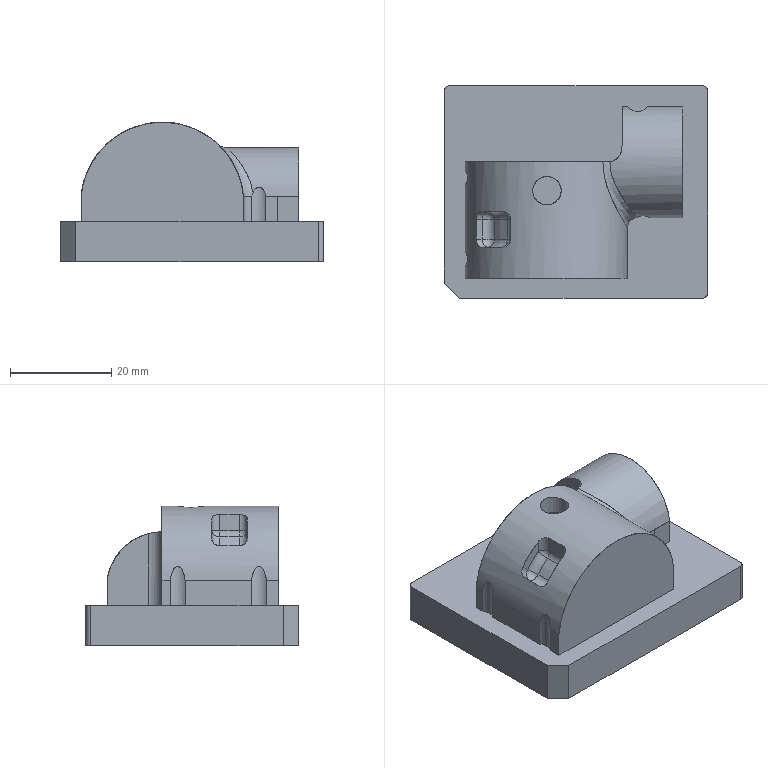NC program | PowerMill | posted with a generic post | part box 52 x 42 x 27.622 mm
Lines 35812 to 36533 of 214543:
N35909 M6
N35910 S8500 M03
N35911 G00 G90 X0.0 Y0.0
N35912 G43 Z9.8022 H3
N35913
N35914 G05 P10000 R8
N35915 X-31.7585 Y-27.2674
N35916 Z-18.62
N35917 G01 Z-19.82 F360.0
N35918 X-28.0283 Y-23.5376 F600.0
N35919 X-25.5003 Y-21.0097
N35920 X-25.7421 Y-20.7679
N35921 X-26.034 Y-20.4345
N35922 G02 X-26.4761 Y-19.7862 I4.9869 J3.8747
N35923 G02 X-26.8165 Y-19.0792 I5.3616 J3.0176
N35924 G01 X-26.9462 Y-18.7087
N35925 X-27.0478 Y-18.3294
N35926 X-27.1208 Y-17.9437
N35927 X-27.1647 Y-17.5535
N35928 X-27.1794 Y-17.1612
N35929 Y-14.7229
N35930 X-27.1661 Y-14.3483
N35931 X-27.126 Y-13.9757
N35932 X-27.0832 Y-13.7323
N35933 X-27.0299 Y-13.4909
N35934 G03 X-27.0298 Y-12.9964 I-0.9689 J0.2473
N35935 G02 X-27.1534 Y-12.257 I4.4498 J1.1234
N35936 G01 X-27.1661 Y-12.139
N35937 X-27.1794 Y-11.7644
N35938 Y1.3491
N35939 X-27.1661 Y1.7237
N35940 X-27.126 Y2.0963
N35941 X-27.0594 Y2.4652
N35942 X-27.0299 Y2.581
N35943 G03 Y3.0757 I-0.9689 J0.2473
N35944 G01 X-27.0826 Y3.3199
N35945 X-27.126 Y3.5604
N35946 X-27.1661 Y3.933
N35947 X-27.1794 Y4.3076
N35948 Y5.9414
N35949 X-27.1647 Y6.3337
N35950 X-27.1208 Y6.7239
N35951 X-27.0478 Y7.1096
N35952 X-26.9462 Y7.4889
N35953 X-26.8165 Y7.8594
N35954 G02 X-26.4952 Y8.5301 I5.2353 J-2.0955
N35955 G01 X-26.2672 Y8.8988
N35956 X-26.0341 Y9.2147
N35957 X-25.778 Y9.5123
N35958 X-25.5003 Y9.7899
N35959 X-25.2028 Y10.046
N35960 X-24.8869 Y10.2792
N35961 X-24.5544 Y10.488
N35962 X-24.2073 Y10.6715
N35963 X-23.9315 Y10.7922
N35964 X-23.6503 Y10.8995
N35965 X-24.9728 Y15.5253
N35966 X-25.4378 Y15.3924
N35967 G02 X-26.5431 Y16.2689 I-0.2386 J0.8343
N35968 G01 X-26.389 Y19.4393
N35969 G02 X-24.2172 Y21.5109 I2.1749 J-0.1058
N35970 G01 X-0.9855 Y21.5443
N35971 G02 X-0.1644 Y20.419 I0.0012 J-0.8614
N35972 G01 X-0.2657 Y20.1041
N35973 G03 X-0.77 Y17.8703 I12.1965 J-3.9269
N35974 G01 X-0.8682 Y17.1333
N35975 G02 X-2.1661 Y15.9958 I-1.2992 J0.1732
N35976 G01 X-22.4475 Y15.9761
N35977 X-22.832 Y15.9498
N35978 G03 X-24.6938 Y15.6051 I0.8699 J-9.8993
N35979 G01 X-24.9728 Y15.5253
N35980 X-23.6503 Y10.8995
N35981 X-23.4769 Y10.9581
N35982 G02 X-22.7119 Y11.1328 I1.7411 J-5.8651
N35983 G01 X-22.3218 Y11.1767
N35984 X-21.9294 Y11.1914
N35985 X2.8992
N35986 G03 X3.899 Y12.1739 I0.0 J1.0
N35987 G01 X3.9812 Y16.8798
N35988 X4.0023 Y17.2674
N35989 X4.052 Y17.6525
N35990 X4.1301 Y18.0328
N35991 X4.236 Y18.4063
N35992 X4.3692 Y18.771
N35993 X4.5291 Y19.1248
N35994 X4.7146 Y19.4659
N35995 X4.9248 Y19.7922
N35996 G02 X5.4147 Y20.3941 I4.9294 J-3.5117
N35997 G01 X5.6916 Y20.6662
N35998 X5.9878 Y20.9171
N35999 X6.3018 Y21.1455
N36000 X6.6319 Y21.35
N36001 X6.9761 Y21.5295
N36002 X7.3327 Y21.6832
N36003 X7.6996 Y21.81
N36004 X8.0749 Y21.9094
N36005 G02 X8.8424 Y22.0238 I1.2982 J-6.0795
N36006 G01 X9.2304 Y22.0381
N36007 X10.4243 Y22.0338
N36008 X10.6703 Y22.0233
N36009 X11.0623 Y21.9789
N36010 X11.45 Y21.9052
N36011 X11.8713 Y21.7884
N36012 G03 X12.5351 I0.3319 J0.9433
N36013 G01 X12.9565 Y21.9052
N36014 X13.3441 Y21.9789
N36015 X13.7362 Y22.0233
N36016 X14.1305 Y22.0381
N36017 X21.0985
N36018 X21.4909 Y22.0234
N36019 X21.881 Y21.9795
N36020 X22.2668 Y21.9065
N36021 X22.646 Y21.8049
N36022 X23.0166 Y21.6752
N36023 X23.4171 Y21.4968
N36024 X23.7235 Y21.3348
N36025 X24.056 Y21.1259
N36026 X24.3719 Y20.8927
N36027 X24.6694 Y20.6367
N36028 X24.9471 Y20.359
N36029 X25.2031 Y20.0615
N36030 X25.4363 Y19.7456
N36031 X25.6452 Y19.4131
N36032 G02 X26.0006 Y18.6635 I-4.9294 J-2.7961
N36033 G01 X26.1153 Y18.3356
N36034 X26.2169 Y17.9564
N36035 X26.2899 Y17.5706
N36036 X26.3339 Y17.1805
N36037 X26.3485 Y16.7881
N36038 Y-5.1044
N36039 X26.3338 Y-5.4968
N36040 X26.2899 Y-5.8869
N36041 X26.2169 Y-6.2727
N36042 X26.1153 Y-6.6519
N36043 X25.9856 Y-7.0225
N36044 X25.8286 Y-7.3823
N36045 X25.6452 Y-7.7294
N36046 X25.4363 Y-8.0619
N36047 X25.2031 Y-8.3778
N36048 X24.947 Y-8.6753
N36049 X24.6694 Y-8.9529
N36050 X24.3718 Y-9.2091
N36051 X24.056 Y-9.4422
N36052 X23.7235 Y-9.6511
N36053 X23.3764 Y-9.8345
N36054 X23.1798 Y-9.9203
N36055 X24.9239 Y-14.3937
N36056 X25.448 Y-14.1894
N36057 G02 X26.5446 Y-14.9628 I0.2923 J-0.7497
N36058 G01 X26.4152 Y-19.3477
N36059 G02 X24.1935 Y-21.5191 I-2.2365 J0.0661
N36060 G01 X20.5691 Y-21.5432
N36061 G02 X19.7114 Y-20.4389 I-0.0058 J0.8807
N36062 G01 X19.9263 Y-19.62
N36063 G03 X20.2939 Y-16.7253 I-10.8588 J2.8496
N36064 G01 X20.2926 Y-16.4098
N36065 G02 X21.3497 Y-15.2059 I1.2086 J0.0048
N36066 G01 X22.2848 Y-15.0878
N36067 G03 X24.7492 Y-14.4618 I-1.2987 J10.2777
N36068 G01 X24.9239 Y-14.3937
N36069 X23.1798 Y-9.9203
N36070 X23.0166 Y-9.9915
N36071 X22.646 Y-10.1212
N36072 X22.2668 Y-10.2228
N36073 G02 X21.4909 Y-10.3398 I-1.2879 J5.912
N36074 G01 X21.0985 Y-10.3544
N36075 X16.4239
N36076 G03 X15.4239 Y-11.3544 I0.0 J-1.0
N36077 G01 Y-17.1612
N36078 X15.4092 Y-17.5535
N36079 X15.3652 Y-17.9437
N36080 X15.2922 Y-18.3294
N36081 X15.1906 Y-18.7087
N36082 X15.061 Y-19.0792
N36083 X14.904 Y-19.4391
N36084 X14.7205 Y-19.7862
N36085 X14.4841 Y-20.1559
N36086 X14.2785 Y-20.4345
N36087 X14.0224 Y-20.7321
N36088 X13.7448 Y-21.0097
N36089 X13.4472 Y-21.2658
N36090 X13.1313 Y-21.499
N36091 X12.7989 Y-21.7078
N36092 X12.4518 Y-21.8913
N36093 X12.0919 Y-22.0483
N36094 X11.7214 Y-22.1779
N36095 X11.3421 Y-22.2796
N36096 X10.9564 Y-22.3526
N36097 X10.5662 Y-22.3965
N36098 X10.1739 Y-22.4112
N36099 X-21.9294
N36100 X-22.3218 Y-22.3965
N36101 X-22.7119 Y-22.3526
N36102 X-23.0977 Y-22.2796
N36103 X-23.4769 Y-22.1779
N36104 X-23.8475 Y-22.0483
N36105 X-24.2073 Y-21.8913
N36106 X-24.5544 Y-21.7078
N36107 X-24.8869 Y-21.4989
N36108 X-25.2028 Y-21.2658
N36109 X-25.5003 Y-21.0097
N36110 X-28.0283 Y-23.5376
N36111 G00 Z9.8022
N36112 G05 P0
N36113 (---------------)
N36114 ( END TOOLPATH : 粗公基准台01-基准面偏置-D10 )
N36115 (---------------)
N36116 ( START TOOLPATH : 粗公基准台01-外形侧光-D10 )
N36117 (---------------)
N36118 G00 X0.0 Y0.0 Z10.802
N36119 G05 P10000 R8
N36120 X26.0718 Y16.531
N36121 Z-8.294
N36122 G01 Z-9.494 F360.0
N36123 G03 X25.8674 Y15.4013 I1.2615 J-0.8115 F600.0
N36124 G02 X25.9777 Y14.4568 I-4.7691 J-1.0354
N36125 G01 X25.9785 Y-2.5824
N36126 G02 X25.8673 Y-3.72 I-4.8822 J-0.0969
N36127 G03 X26.0705 Y-4.8499 I1.4655 J-0.3196
N36128 G00 Z4.1556
N36129 G01 X10.7901 Y-22.1365 F10000.0
N36130 G00 Z-8.294
N36131 G01 Z-9.494 F360.0
N36132 G03 X9.6606 Y-21.9311 I-0.8127 J-1.2607 F600.0
N36133 G02 X8.6481 Y-22.0412 I-1.0309 J4.77
N36134 G01 X-5.8084
N36135 X-20.2656
N36136 G02 X-21.4209 Y-21.9306 I-0.1155 J4.8832
N36137 G03 X-22.5508 Y-22.1341 I-0.3194 J-1.4656
N36138 G00 Z4.1556
N36139 G01 X-22.5476 Y10.9144 F10000.0
N36140 G00 Z-8.294
N36141 G01 Z-9.494 F360.0
N36142 G03 X-21.4177 Y10.7107 I0.8108 J1.262 F600.0
N36143 G02 X-20.2649 Y10.8214 I1.041 J-4.7825
N36144 G01 X4.029
N36145 G03 X4.249 Y11.0376 I0.0 J0.22
N36146 G01 X4.3083 Y14.4602
N36147 G02 X4.4379 Y15.4867 I4.8792 J-0.0944
N36148 G03 X4.2539 Y16.6199 I-1.4599 J0.3445
N36149 G00 Z4.1556
N36150 G01 X26.1834 Y16.0152 F10000.0
N36151 G00 Z-8.294
N36152 G01 Z-9.494 F360.0
N36153 G03 X25.8674 Y14.9115 I1.1743 J-0.9332 F600.0
N36154 G02 X25.8977 Y14.4565 I-4.7687 J-0.5455
N36155 G01 X25.8985 Y-2.5815
N36156 G02 X25.8673 Y-3.2346 I-4.8024 J-0.0978
N36157 G03 X26.1811 Y-4.339 I1.49 J-0.1734
N36158 G00 Z4.1556
N36159 G01 X10.2699 Y-22.249 F10000.0
N36160 G00 Z-8.294
N36161 G01 Z-9.494 F360.0
N36162 G03 X9.1667 Y-21.9311 I-0.9354 J-1.1727 F600.0
N36163 G02 X8.6481 Y-21.9612 I-0.5369 J4.7706
N36164 G01 X-5.8084
N36165 X-20.2649
N36166 G02 X-20.9346 Y-21.9306 I-0.1162 J4.8032
N36167 G03 X-22.0388 Y-22.2448 I-0.1728 J-1.49
N36168 G00 Z4.1556
N36169 G01 X-22.0348 Y11.0251 F10000.0
N36170 G00 Z-8.294
N36171 G01 Z-9.494 F360.0
N36172 G03 X-20.9306 Y10.7107 I0.9316 J1.1756 F600.0
N36173 G02 X-20.2649 Y10.7414 I0.5539 J-4.7828
N36174 G01 X4.029
N36175 G03 X4.329 Y11.0362 I0.0 J0.3
N36176 G01 X4.3882 Y14.4565
N36177 G02 X4.4292 Y14.9985 I4.7991 J-0.0906
N36178 G03 X4.1335 Y16.1078 I-1.4869 J0.1977
N36179 G00 Z4.1889
N36180 G01 X15.4933 Y-12.0436 F10000.0
N36181 G00 Z-18.59
N36182 G01 Z-19.79 F360.0
N36183 G03 X15.0539 Y-13.1043 I1.0606 J-1.0607 F600.0
N36184 G01 Y-17.0386
N36185 G02 X10.197 Y-22.0411 I-4.883 J-0.1182
N36186 G01 X-5.8084 Y-22.0412
N36187 X-21.8145
N36188 G02 X-26.8075 Y-17.2968 I-0.1109 J4.8828
N36189 G02 X-26.8094 Y-14.7124 I174.8409 J1.418
N36190 G02 X-26.5991 Y-13.3087 I4.7813 J0.0012
N36191 G03 X-26.5975 Y-13.1867 I-0.2105 J0.0636
N36192 G02 X-26.8082 Y-11.8754 I4.669 J1.4225
N36193 G01 X-26.8094 Y1.292
N36194 G02 X-26.599 Y2.7658 I4.881 J0.0548
N36195 G03 X-26.5979 Y2.8926 I-0.2101 J0.0651
N36196 G02 X-26.8062 Y4.1294 I4.5302 J1.3987
N36197 G02 X-26.8094 Y5.9396 I71.3503 J1.0334
N36198 G02 X-21.8139 Y10.8214 I4.8839 J-0.0008
N36199 G01 X4.029
N36200 G03 X4.249 Y11.0376 I0.0 J0.22
N36201 G01 X4.3183 Y15.0005
N36202 X4.3495 Y16.7822
N36203 G02 X9.1644 Y21.6677 I4.8827 J0.0032
N36204 G02 X10.4603 Y21.6646 I0.5369 J-47.0757
N36205 G02 X12.1196 Y21.3052 I-0.1677 J-4.7838
N36206 G03 X12.2831 Y21.3036 I0.0838 J0.2034
N36207 G02 X14.0693 Y21.6678 I1.8403 J-4.4639
N36208 G01 X15.0759
N36209 X21.0407 Y21.6681
N36210 G02 X25.9785 Y16.7799 I0.0568 J-4.8807
N36211 G01 X25.9781 Y-5.1662
N36212 G02 X21.0394 Y-9.9844 I-4.8807 J0.0625
N36213 G01 X15.2739
N36214 G03 X15.0539 Y-10.2044 I0.0 J-0.22
N36215 G01 Y-13.1043
N36216 G03 X15.4933 Y-14.165 I1.5 J0.0
N36217 G01 X15.4133 Y-11.9768
N36218 G03 X14.9739 Y-13.0375 I1.0606 J-1.0607
N36219 G01 Y-17.038
N36220 G02 X10.197 Y-21.9611 I-4.8029 J-0.1188
N36221 G01 X-5.8084 Y-21.9612
N36222 X-21.8139
N36223 G02 X-26.7275 Y-17.2962 I-0.1115 J4.8028
N36224 G02 X-26.7294 Y-14.7147 I174.7309 J1.4187
N36225 G02 X-26.5225 Y-13.3319 I4.7004 J0.0035
N36226 G03 X-26.5204 Y-13.1655 I-0.2872 J0.0868
N36227 G02 X-26.7282 Y-11.875 I4.5906 J1.4011
N36228 G01 X-26.7294 Y1.2908
N36229 G02 X-26.5225 Y2.7421 I4.8006 J0.056
N36230 G03 X-26.5211 Y2.915 I-0.2866 J0.0888
N36231 G02 X-26.7262 Y4.1304 I4.4521 J1.3761
N36232 G02 X-26.7294 Y5.9375 I71.1887 J1.0327
N36233 G02 X-21.8139 Y10.7414 I4.8039 J0.0013
N36234 G01 X4.029
N36235 G03 X4.329 Y11.0362 I0.0 J0.3
N36236 G01 X4.3983 Y14.9991
N36237 X4.4295 Y16.7799
N36238 G02 X9.1644 Y21.5877 I4.8027 J0.0055
N36239 G02 X10.4552 Y21.5848 I0.5372 J-48.3015
N36240 G02 X12.0891 Y21.2312 I-0.1625 J-4.7033
N36241 G03 X12.3121 Y21.229 I0.1143 J0.2774
N36242 G02 X14.0693 Y21.5878 I1.8111 J-4.3881
N36243 G01 X15.0759
N36244 X21.0394 Y21.5881
N36245 G02 X25.8985 Y16.7799 I0.0581 J-4.8007
N36246 G01 X25.8982 Y-5.163
N36247 G02 X21.0394 Y-9.9044 I-4.8007 J0.0593
N36248 G01 X15.2739
N36249 G03 X14.9739 Y-10.2044 I0.0 J-0.3
N36250 G01 Y-13.0375
N36251 G03 X15.4133 Y-14.0982 I1.5 J0.0
N36252 G00 Z10.802
N36253 G05 P0
N36254 (---------------)
N36255 ( END TOOLPATH : 粗公基准台01-外形侧光-D10 )
N36256 (---------------)
N36257 ( START TOOLPATH : 粗公基准台01-基准台侧光-D10 )
N36258 (---------------)
N36259 G00 X0.0 Y0.0 Z9.8022
N36260 G05 P10000 R8
N36261 X31.5194 Y-28.9518
N36262 Z-26.52
N36263 G01 Z-27.72 F360.0
N36264 G03 X28.4722 Y-24.9877 I-1.5236 J1.982 F600.0
N36265 G01 X28.4323 Y-25.0183
N36266 X28.429 Y-25.0208
N36267 X28.4255 Y-25.023
N36268 X27.9786 Y-25.2983
N36269 X27.9758 Y-25.2999
N36270 X27.973 Y-25.3014
N36271 X27.526 Y-25.5298
N36272 X27.5229 Y-25.5313
N36273 X27.5198 Y-25.5327
N36274 X27.0728 Y-25.7144
N36275 X27.0699 Y-25.7155
N36276 X27.067 Y-25.7165
N36277 X26.62 Y-25.8596
N36278 X26.6171 Y-25.8605
N36279 X26.614 Y-25.8613
N36280 X26.1671 Y-25.9669
N36281 X26.1648 Y-25.9674
N36282 X26.1626 Y-25.9678
N36283 X25.958 Y-26.0039
N36284 X25.9565 Y-26.0042
N36285 X25.955 Y-26.0044
N36286 X25.7125 Y-26.0376
N36287 X25.7102 Y-26.0379
N36288 X25.708 Y-26.0381
N36289 X25.261 Y-26.0733
N36290 X25.2584 Y-26.0734
N36291 X25.2558 Y-26.0735
N36292 X24.8089 Y-26.08
N36293 X24.8083
N36294 X24.8077
N36295 X-23.0198
N36296 X-23.0217
N36297 X-23.0237 Y-26.0799
N36298 X-23.4706 Y-26.0581
N36299 X-23.474 Y-26.0578
N36300 X-23.4774 Y-26.0575
N36301 X-23.8725 Y-26.0045
N36302 X-23.8761 Y-26.0039
N36303 X-23.8797 Y-26.0032
N36304 X-24.3785 Y-25.8893
N36305 X-24.3823 Y-25.8883
N36306 X-24.3861 Y-25.8872
N36307 X-24.8331 Y-25.7377
N36308 X-24.8366 Y-25.7364
N36309 X-24.84 Y-25.735
N36310 X-25.2562 Y-25.5514
N36311 X-25.2599 Y-25.5497
N36312 X-25.2634 Y-25.5478
N36313 X-25.7411 Y-25.2768
N36314 X-25.7441 Y-25.2751
N36315 X-25.747 Y-25.2732
N36316 X-26.0033 Y-25.0971
N36317 X-26.0051 Y-25.0959
N36318 X-26.0068 Y-25.0945
N36319 X-26.1975 Y-24.9474
N36320 X-26.1997 Y-24.9457
N36321 X-26.2018 Y-24.9439
N36322 X-26.5393 Y-24.644
N36323 X-26.5411 Y-24.6424
N36324 X-26.5428 Y-24.6408
N36325 X-29.6706 Y-21.5119
N36326 X-29.6716 Y-21.5108
N36327 X-29.6727 Y-21.5096
N36328 X-29.7833 Y-21.3902
N36329 X-29.7848 Y-21.3884
N36330 X-29.7863 Y-21.3866
N36331 X-30.0556 Y-21.0591
N36332 X-30.0574 Y-21.0568
N36333 X-30.0591 Y-21.0545
N36334 X-30.2369 Y-20.8027
N36335 X-30.2381 Y-20.8009
N36336 X-30.2393 Y-20.7991
N36337 X-30.3619 Y-20.6039
N36338 X-30.3634 Y-20.6014
N36339 X-30.3648 Y-20.5988
N36340 X-30.6017 Y-20.1518
N36341 X-30.603 Y-20.1492
N36342 X-30.6042 Y-20.1466
N36343 X-30.6917 Y-19.9478
N36344 X-30.6925 Y-19.946
N36345 X-30.6932 Y-19.9442
N36346 X-30.7885 Y-19.6961
N36347 X-30.7895 Y-19.6933
N36348 X-30.7904 Y-19.6905
N36349 X-30.9254 Y-19.2435
N36350 X-30.9264 Y-19.2399
N36351 X-30.9272 Y-19.2364
N36352 X-31.0182 Y-18.7894
N36353 X-31.0189 Y-18.7858
N36354 X-31.0194 Y-18.7822
N36355 X-31.0689 Y-18.3352
N36356 X-31.0692 Y-18.3318
N36357 X-31.0693 Y-18.3283
N36358 X-31.08 Y-17.8813
N36359 Y-17.8804
N36360 Y-17.8794
N36361 Y19.2204
N36362 Y19.2205
N36363 X-31.0787 Y20.1145
N36364 Y20.1168
N36365 X-31.0786 Y20.1191
N36366 X-31.052 Y20.5661
N36367 X-31.0518 Y20.5688
N36368 X-31.0514 Y20.5716
N36369 X-30.9937 Y21.0186
N36370 X-30.9932 Y21.0218
N36371 X-30.9926 Y21.025
N36372 X-30.8977 Y21.4719
N36373 X-30.897 Y21.4748
N36374 X-30.8963 Y21.4775
N36375 X-30.767 Y21.9245
N36376 X-30.766 Y21.9276
N36377 X-30.7649 Y21.9306
N36378 X-30.5958 Y22.3776
N36379 X-30.5945 Y22.3807
N36380 X-30.5932 Y22.3837
N36381 X-30.3803 Y22.8307
N36382 X-30.3788 Y22.8336
N36383 X-30.3772 Y22.8365
N36384 X-30.1168 Y23.2835
N36385 X-30.1149 Y23.2866
N36386 X-30.1129 Y23.2896
N36387 X-29.7948 Y23.7366
N36388 X-29.7924 Y23.7398
N36389 X-29.7899 Y23.7429
N36390 X-29.3378 Y24.2601
N36391 X-29.3348 Y24.2633
N36392 X-29.3316 Y24.2664
N36393 X-28.9198 Y24.6432
N36394 X-28.9173 Y24.6455
N36395 X-28.9146 Y24.6476
N36396 X-28.4323 Y25.0183
N36397 X-28.429 Y25.0208
N36398 X-28.4255 Y25.023
N36399 X-27.9786 Y25.2983
N36400 X-27.9758 Y25.2999
N36401 X-27.973 Y25.3014
N36402 X-27.526 Y25.5298
N36403 X-27.5229 Y25.5313
N36404 X-27.5198 Y25.5327
N36405 X-27.0728 Y25.7144
N36406 X-27.0699 Y25.7155
N36407 X-27.067 Y25.7165
N36408 X-26.62 Y25.8596
N36409 X-26.6171 Y25.8605
N36410 X-26.614 Y25.8613
N36411 X-26.167 Y25.9669
N36412 X-26.164 Y25.9675
N36413 X-26.1609 Y25.9681
N36414 X-25.7139 Y26.0374
N36415 X-25.711 Y26.0378
N36416 X-25.708 Y26.0381
N36417 X-25.261 Y26.0733
N36418 X-25.2584 Y26.0735
N36419 X-25.2558
N36420 X-24.8089 Y26.08
N36421 X-24.8083
N36422 X-24.8077
N36423 X0.0
N36424 X24.8077
N36425 X24.8083
N36426 X24.8089
N36427 X25.2558 Y26.0735
N36428 X25.2584
N36429 X25.261 Y26.0733
N36430 X25.708 Y26.0381
N36431 X25.711 Y26.0378
N36432 X25.7139 Y26.0374
N36433 X26.1609 Y25.9681
N36434 X26.164 Y25.9675
N36435 X26.1671 Y25.9669
N36436 X26.614 Y25.8613
N36437 X26.6171 Y25.8605
N36438 X26.62 Y25.8596
N36439 X27.067 Y25.7165
N36440 X27.0698 Y25.7156
N36441 X27.0725 Y25.7146
N36442 X27.4761 Y25.5524
N36443 X27.4793 Y25.5511
N36444 X27.4824 Y25.5496
N36445 X27.9727 Y25.3016
N36446 X27.9757 Y25.3
N36447 X27.9786 Y25.2983
N36448 X28.4255 Y25.023
N36449 X28.4289 Y25.0208
N36450 X28.4321 Y25.0185
N36451 X28.8791 Y24.6776
N36452 X28.8818 Y24.6755
N36453 X28.8844 Y24.6732
N36454 X29.3314 Y24.2666
N36455 X29.3347 Y24.2634
N36456 X29.3378 Y24.2601
N36457 X29.7847 Y23.7493
N36458 X29.7873 Y23.7463
N36459 X29.7897 Y23.7431
N36460 X30.1128 Y23.2897
N36461 X30.1149 Y23.2866
N36462 X30.1168 Y23.2835
N36463 X30.3772 Y22.8365
N36464 X30.3788 Y22.8336
N36465 X30.3803 Y22.8307
N36466 X30.5932 Y22.3837
N36467 X30.5945 Y22.3807
N36468 X30.5958 Y22.3776
N36469 X30.7649 Y21.9306
N36470 X30.766 Y21.9276
N36471 X30.767 Y21.9245
N36472 X30.8962 Y21.4775
N36473 X30.897 Y21.4747
N36474 X30.8976 Y21.4719
N36475 X30.9926 Y21.025
N36476 X30.9932 Y21.0218
N36477 X30.9937 Y21.0186
N36478 X31.0514 Y20.5716
N36479 X31.0517 Y20.5688
N36480 X31.052 Y20.5661
N36481 X31.0786 Y20.1191
N36482 X31.0787 Y20.1168
N36483 Y20.1146
N36484 X31.08 Y19.6676
N36485 Y19.6675
N36486 Y19.6674
N36487 Y-19.2204
N36488 Y-19.2205
N36489 X31.0787 Y-20.1145
N36490 Y-20.1168
N36491 X31.0786 Y-20.1191
N36492 X31.0519 Y-20.5661
N36493 X31.0517 Y-20.5688
N36494 X31.0514 Y-20.5716
N36495 X30.9937 Y-21.0186
N36496 X30.9932 Y-21.0218
N36497 X30.9926 Y-21.0249
N36498 X30.8977 Y-21.4719
N36499 X30.897 Y-21.4748
N36500 X30.8962 Y-21.4775
N36501 X30.7669 Y-21.9245
N36502 X30.766 Y-21.9276
N36503 X30.7649 Y-21.9306
N36504 X30.5958 Y-22.3776
N36505 X30.5945 Y-22.3807
N36506 X30.5932 Y-22.3837
N36507 X30.3803 Y-22.8307
N36508 X30.3788 Y-22.8336
N36509 X30.3772 Y-22.8365
N36510 X30.1168 Y-23.2835
N36511 X30.1149 Y-23.2866
N36512 X30.1129 Y-23.2896
N36513 X29.7948 Y-23.7366
N36514 X29.7924 Y-23.7398
N36515 X29.7899 Y-23.7429
N36516 X29.3378 Y-24.2601
N36517 X29.3348 Y-24.2633
N36518 X29.3316 Y-24.2664
N36519 X28.9198 Y-24.6432
N36520 X28.9173 Y-24.6455
N36521 X28.9146 Y-24.6476
N36522 X28.4722 Y-24.9877
N36523 G03 X31.5194 Y-28.9519 I1.5236 J-1.9821
N36524 G01 X31.4681 Y-28.8903
N36525 G03 X28.421 Y-24.9262 I-1.5236 J1.982
N36526 G01 X28.3836 Y-24.9549
N36527 X27.9366 Y-25.2302
N36528 X27.4896 Y-25.4586
N36529 X27.0426 Y-25.6403
N36530 X26.5956 Y-25.7834
N36531 X26.1487 Y-25.889
N36532 X25.9441 Y-25.9252
N36533 X25.7017 Y-25.9584
N36534 X25.2547 Y-25.9935
N36535 X24.8077 Y-26.0
N36536 X-23.0198
N36537 X-23.4667 Y-25.9782
N36538 X-23.8619 Y-25.9252
N36539 X-24.3607 Y-25.8113
N36540 X-24.8077 Y-25.6618
N36541 X-25.2239 Y-25.4782
N36542 X-25.7017 Y-25.2073
N36543 X-25.958 Y-25.0312
N36544 X-26.1487 Y-24.8841
N36545 X-26.4862 Y-24.5842
N36546 X-29.614 Y-21.4553
N36547 X-29.7245 Y-21.3358
N36548 X-29.9938 Y-21.0083
N36549 X-30.1715 Y-20.7565
N36550 X-30.2941 Y-20.5613
N36551 X-30.531 Y-20.1144
N36552 X-30.6185 Y-19.9156
N36553 X-30.7138 Y-19.6674
N36554 X-30.8488 Y-19.2204
N36555 X-30.9399 Y-18.7734
N36556 X-30.9894 Y-18.3264
N36557 X-31.0 Y-17.8794
N36558 Y19.2204
N36559 X-30.9987 Y20.1144
N36560 X-30.9721 Y20.5613
N36561 X-30.9144 Y21.0083
N36562 X-30.8194 Y21.4553
N36563 X-30.6901 Y21.9023
N36564 X-30.5209 Y22.3493
N36565 X-30.3081 Y22.7963
N36566 X-30.0477 Y23.2433
N36567 X-29.7296 Y23.6902
N36568 X-29.2776 Y24.2074
N36569 X-28.8658 Y24.5842
N36570 X-28.3836 Y24.9549
N36571 X-27.9366 Y25.2302
N36572 X-27.4896 Y25.4586
N36573 X-27.0426 Y25.6403
N36574 X-26.5956 Y25.7835
N36575 X-26.1487 Y25.889
N36576 X-25.7017 Y25.9584
N36577 X-25.2547 Y25.9935
N36578 X-24.8077 Y26.0
N36579 X0.0
N36580 X24.8077
N36581 X25.2547 Y25.9936
N36582 X25.7017 Y25.9584
N36583 X26.1487 Y25.889
N36584 X26.5956 Y25.7834
N36585 X27.0426 Y25.6403
N36586 X27.4463 Y25.4782
N36587 X27.9366 Y25.2302
N36588 X28.3836 Y24.9549
N36589 X28.8306 Y24.614
N36590 X29.2776 Y24.2074
N36591 X29.7245 Y23.6966
N36592 X30.0477 Y23.2433
N36593 X30.3081 Y22.7963
N36594 X30.5209 Y22.3493
N36595 X30.6901 Y21.9023
N36596 X30.8194 Y21.4553
N36597 X30.9143 Y21.0083
N36598 X30.9721 Y20.5613
N36599 X30.9987 Y20.1144
N36600 X31.0 Y19.6674
N36601 Y-19.2204
N36602 X30.9987 Y-20.1144
N36603 X30.9721 Y-20.5613
N36604 X30.9143 Y-21.0083
N36605 X30.8194 Y-21.4553
N36606 X30.6901 Y-21.9023
N36607 X30.5209 Y-22.3493
N36608 X30.3081 Y-22.7963
N36609 X30.0477 Y-23.2433
N36610 X29.7296 Y-23.6902
N36611 X29.2776 Y-24.2074
N36612 X28.8658 Y-24.5842
N36613 X28.421 Y-24.9262
N36614 G03 X31.4681 Y-28.8903 I1.5236 J-1.9821
N36615 G00 Z9.8022
N36616 G05 P0
N36617 (---------------)
N36618 ( END TOOLPATH : 粗公基准台01-基准台侧光-D10 )
N36619 (---------------)
N36620
N36621 M05
N36622 G53 Z0.0
N36623 (---------------)
N36624 ( START TOOLPATH : 粗公精光01-平行-R2 )
N36625 (---------------)
N36626 ( TOOL NO.    :7 )
N36627 ( TOOL TYPE   : BALLNOSED)
N36628 ( TOOL ID     : R2_2_1)
N36629 ( TOOL DIA    : 4.0 LENGTH 71.6)
N36630 T7